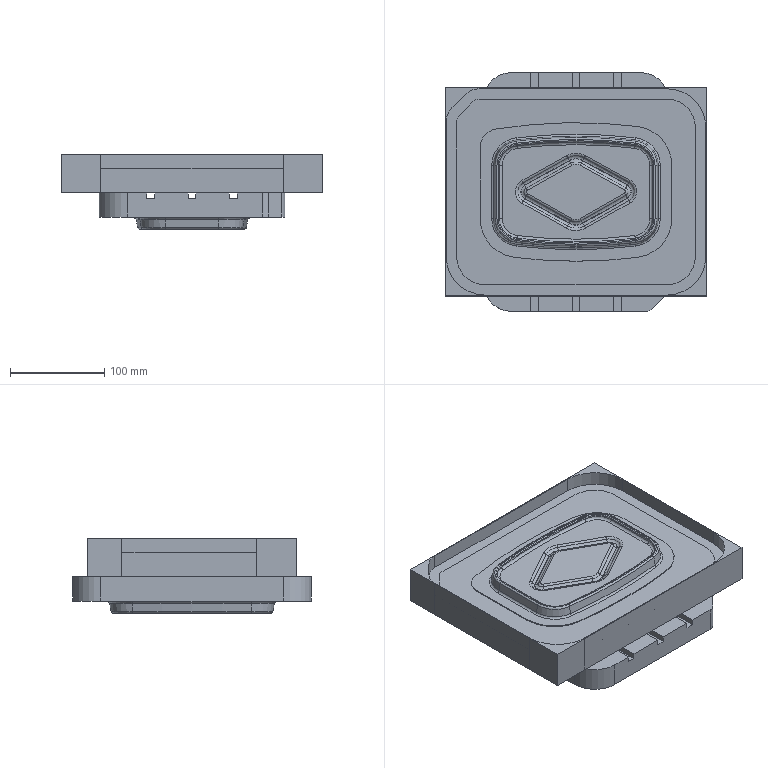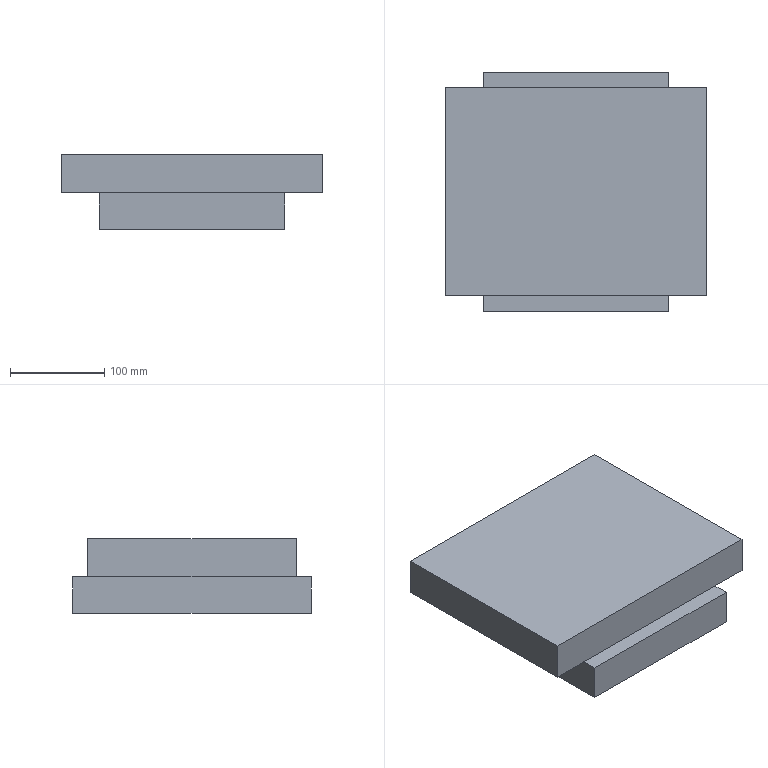CAM job | NX | 3-axis milling, drilling | part box 278.144 x 254.144 x 79 mm | stock box 278.144 x 254.144 x 79 mm
Tools:
number,name,description,diameter,corner_radius,flute_length,length,flutes
0,V2.0,Drilling Tool,2.0,0.0,35.0,50.0,2
0,V8.0,Drilling Tool,8.0,0.0,35.0,50.0,2
0,D10,No Description,10.0,0.0,20.0,60.0,2
0,D4,No Description,4.0,0.0,0.0,20.0,2
0,D8,No Description,8.0,0.0,0.0,40.0,2
0,D16R0.8,No Description,16.0,0.8,50.0,90.0,2
0,R2,No Description,4.0,2.0,0.0,20.0,2
Operations:
program,operation,operation_type,tool,method,geometry_group,spindle_rpm,surface_speed,feed_per_tooth,feed_cut,feed_plunge,cut_length_mm,path_length_mm,cut_time_min,machine_time_min
B-1,CAVITY_MILL_1,CavityMilling,D16R0.8,METHOD,22B,7000.0,1099.0,0.3214,4500.0,100.0,184889.758,187645.411,41.087,41.362
B-2,CAVITY_MILL_1_COPY,CavityMilling,D4,METHOD,22B,7000.0,1099.0,0.3214,4500.0,100.0,21096.264,22552.229,4.688,4.834
B-3,CONTOUR_AREA_1,SurfaceContour,R2,METHOD,22B,8000.0,251.0,0.2812,4500.0,100.0,120992.923,121127.337,26.887,26.901
B-4,DRILLING,Operation,V2.0,METHOD,22B,2000.0,75.0,0.0375,150.0,0.0,235.0,1826.518,1.567,1.726
B-5,FACE_MILLING_1,FaceMilling,D10,METHOD,22B,7000.0,1099.0,0.2857,4000.0,100.0,4881.454,5028.243,1.22,1.235
B-5,PLANAR_MILL_1,PlanarMilling,D10,METHOD,22B,7000.0,571.0,0.2857,4000.0,100.0,31143.21,31316.405,7.786,7.803
C-1,CAVITY_MILL_2,CavityMilling,D8,METHOD,23C,7000.0,1099.0,0.3214,4500.0,100.0,86163.409,111627.474,19.147,21.694
C-2,DRILLING_1,Operation,V2.0,METHOD,23C,2000.0,75.0,0.0375,150.0,0.0,125.0,1034.601,0.8333,0.9243
C-3,DRILLING_1_COPY,Operation,V8.0,METHOD,23C,2000.0,75.0,0.0375,150.0,0.0,225.0,1234.601,1.5,1.601